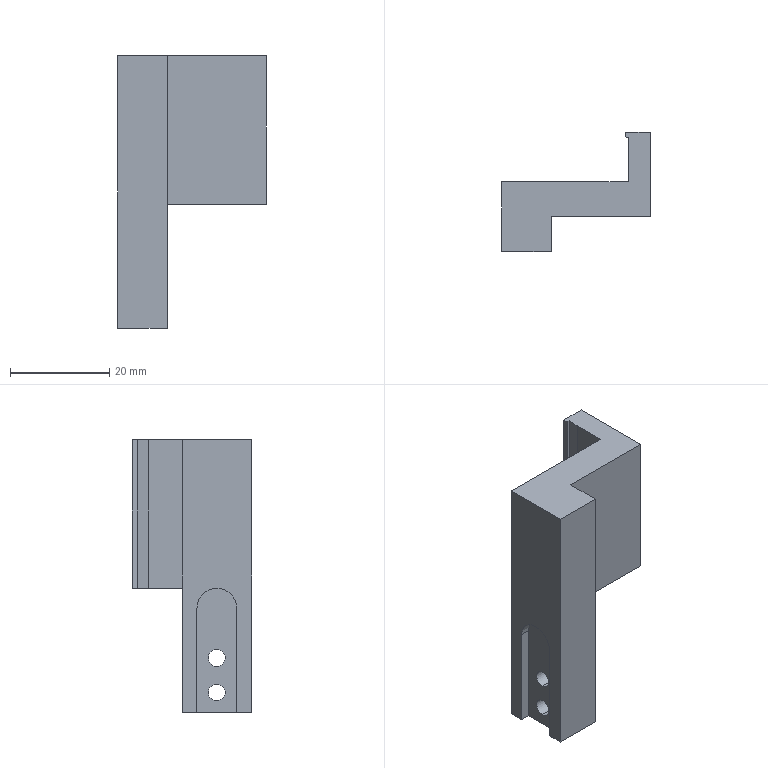Part | STEP file | X77-02303 | 1 solid | 29 faces | box 30 x 24 x 55 mm | volume 12596 mm3 | plane 19 | cylinder 10 | commonest cylinder face diameters 3.4 x4 6 x4 8 x2
STEP:
#1=CARTESIAN_POINT('',(-12.892,-52.894,-18.));
#2=VERTEX_POINT('',#1);
#3=CARTESIAN_POINT('',(-12.892,-52.894,-24.));
#4=VERTEX_POINT('',#3);
#5=CARTESIAN_POINT('',(-12.892,-52.894,-21.));
#6=DIRECTION('',(1.,0.,0.));
#7=DIRECTION('',(0.,0.,-1.));
#8=AXIS2_PLACEMENT_3D('',#5,#6,#7);
#9=CIRCLE('',#8,3.);
#10=EDGE_CURVE('',#2,#4,#9,.T.);
#11=ORIENTED_EDGE('',*,*,#10,.F.);
#12=CARTESIAN_POINT('',(-9.492,-52.894,-18.));
#13=VERTEX_POINT('',#12);
#14=CARTESIAN_POINT('',(-9.492,-52.894,-18.));
#15=DIRECTION('',(1.,0.,0.));
#16=VECTOR('',#15,1000.);
#17=LINE('',#14,#16);
#18=EDGE_CURVE('',#2,#13,#17,.T.);
#19=ORIENTED_EDGE('',*,*,#18,.T.);
#20=CARTESIAN_POINT('',(-9.492,-52.894,-24.));
#21=VERTEX_POINT('',#20);
#22=CARTESIAN_POINT('',(-9.492,-52.894,-21.));
#23=DIRECTION('',(1.,0.,0.));
#24=DIRECTION('',(0.,0.,-1.));
#25=AXIS2_PLACEMENT_3D('',#22,#23,#24);
#26=CIRCLE('',#25,3.);
#27=EDGE_CURVE('',#13,#21,#26,.T.);
#28=ORIENTED_EDGE('',*,*,#27,.T.);
#29=CARTESIAN_POINT('',(-9.492,-52.894,-24.));
#30=DIRECTION('',(1.,0.,0.));
#31=VECTOR('',#30,1000.);
#32=LINE('',#29,#31);
#33=EDGE_CURVE('',#4,#21,#32,.T.);
#34=ORIENTED_EDGE('',*,*,#33,.F.);
#35=EDGE_LOOP('',(#11,#19,#28,#34));
#36=FACE_OUTER_BOUND('',#35,.T.);
#37=CARTESIAN_POINT('',(-9.492,-52.894,-21.));
#38=DIRECTION('',(1.,0.,0.));
#39=DIRECTION('',(0.,0.,-1.));
#40=AXIS2_PLACEMENT_3D('',#37,#38,#39);
#41=CYLINDRICAL_SURFACE('',#40,3.);
#42=ADVANCED_FACE('',(#36),#41,.F.);
#43=CARTESIAN_POINT('',(-17.492,-52.894,-19.3));
#44=VERTEX_POINT('',#43);
#45=CARTESIAN_POINT('',(-17.492,-52.894,-22.7));
#46=VERTEX_POINT('',#45);
#47=CARTESIAN_POINT('',(-17.492,-52.894,-21.));
#48=DIRECTION('',(1.,0.,0.));
#49=DIRECTION('',(0.,0.,-1.));
#50=AXIS2_PLACEMENT_3D('',#47,#48,#49);
#51=CIRCLE('',#50,1.7);
#52=EDGE_CURVE('',#44,#46,#51,.T.);
#53=ORIENTED_EDGE('',*,*,#52,.F.);
#54=CARTESIAN_POINT('',(-12.892,-52.894,-19.3));
#55=VERTEX_POINT('',#54);
#56=CARTESIAN_POINT('',(-9.492,-52.894,-19.3));
#57=DIRECTION('',(1.,0.,0.));
#58=VECTOR('',#57,1000.);
#59=LINE('',#56,#58);
#60=EDGE_CURVE('',#44,#55,#59,.T.);
#61=ORIENTED_EDGE('',*,*,#60,.T.);
#62=CARTESIAN_POINT('',(-12.892,-52.894,-22.7));
#63=VERTEX_POINT('',#62);
#64=CARTESIAN_POINT('',(-12.892,-52.894,-21.));
#65=DIRECTION('',(1.,0.,0.));
#66=DIRECTION('',(0.,0.,-1.));
#67=AXIS2_PLACEMENT_3D('',#64,#65,#66);
#68=CIRCLE('',#67,1.7);
#69=EDGE_CURVE('',#55,#63,#68,.T.);
#70=ORIENTED_EDGE('',*,*,#69,.T.);
#71=CARTESIAN_POINT('',(-9.492,-52.894,-22.7));
#72=DIRECTION('',(1.,0.,0.));
#73=VECTOR('',#72,1000.);
#74=LINE('',#71,#73);
#75=EDGE_CURVE('',#46,#63,#74,.T.);
#76=ORIENTED_EDGE('',*,*,#75,.F.);
#77=EDGE_LOOP('',(#53,#61,#70,#76));
#78=FACE_OUTER_BOUND('',#77,.T.);
#79=CARTESIAN_POINT('',(-9.492,-52.894,-21.));
#80=DIRECTION('',(1.,0.,0.));
#81=DIRECTION('',(0.,0.,-1.));
#82=AXIS2_PLACEMENT_3D('',#79,#80,#81);
#83=CYLINDRICAL_SURFACE('',#82,1.7);
#84=ADVANCED_FACE('',(#78),#83,.F.);
#85=CARTESIAN_POINT('',(-12.892,-52.894,-11.));
#86=VERTEX_POINT('',#85);
#87=CARTESIAN_POINT('',(-12.892,-52.894,-17.));
#88=VERTEX_POINT('',#87);
#89=CARTESIAN_POINT('',(-12.892,-52.894,-14.));
#90=DIRECTION('',(1.,0.,0.));
#91=DIRECTION('',(0.,0.,-1.));
#92=AXIS2_PLACEMENT_3D('',#89,#90,#91);
#93=CIRCLE('',#92,3.);
#94=EDGE_CURVE('',#86,#88,#93,.T.);
#95=ORIENTED_EDGE('',*,*,#94,.F.);
#96=CARTESIAN_POINT('',(-9.492,-52.894,-11.));
#97=VERTEX_POINT('',#96);
#98=CARTESIAN_POINT('',(-9.492,-52.894,-11.));
#99=DIRECTION('',(1.,0.,0.));
#100=VECTOR('',#99,1000.);
#101=LINE('',#98,#100);
#102=EDGE_CURVE('',#86,#97,#101,.T.);
#103=ORIENTED_EDGE('',*,*,#102,.T.);
#104=CARTESIAN_POINT('',(-9.492,-52.894,-17.));
#105=VERTEX_POINT('',#104);
#106=CARTESIAN_POINT('',(-9.492,-52.894,-14.));
#107=DIRECTION('',(1.,0.,0.));
#108=DIRECTION('',(0.,0.,-1.));
#109=AXIS2_PLACEMENT_3D('',#106,#107,#108);
#110=CIRCLE('',#109,3.);
#111=EDGE_CURVE('',#97,#105,#110,.T.);
#112=ORIENTED_EDGE('',*,*,#111,.T.);
#113=CARTESIAN_POINT('',(-9.492,-52.894,-17.));
#114=DIRECTION('',(1.,0.,0.));
#115=VECTOR('',#114,1000.);
#116=LINE('',#113,#115);
#117=EDGE_CURVE('',#88,#105,#116,.T.);
#118=ORIENTED_EDGE('',*,*,#117,.F.);
#119=EDGE_LOOP('',(#95,#103,#112,#118));
#120=FACE_OUTER_BOUND('',#119,.T.);
#121=CARTESIAN_POINT('',(-9.492,-52.894,-14.));
#122=DIRECTION('',(1.,0.,0.));
#123=DIRECTION('',(0.,0.,-1.));
#124=AXIS2_PLACEMENT_3D('',#121,#122,#123);
#125=CYLINDRICAL_SURFACE('',#124,3.);
#126=ADVANCED_FACE('',(#120),#125,.F.);
#127=CARTESIAN_POINT('',(-17.492,-52.894,-12.3));
#128=VERTEX_POINT('',#127);
#129=CARTESIAN_POINT('',(-17.492,-52.894,-15.7));
#130=VERTEX_POINT('',#129);
#131=CARTESIAN_POINT('',(-17.492,-52.894,-14.));
#132=DIRECTION('',(1.,0.,0.));
#133=DIRECTION('',(0.,0.,-1.));
#134=AXIS2_PLACEMENT_3D('',#131,#132,#133);
#135=CIRCLE('',#134,1.7);
#136=EDGE_CURVE('',#128,#130,#135,.T.);
#137=ORIENTED_EDGE('',*,*,#136,.F.);
#138=CARTESIAN_POINT('',(-12.892,-52.894,-12.3));
#139=VERTEX_POINT('',#138);
#140=CARTESIAN_POINT('',(-9.492,-52.894,-12.3));
#141=DIRECTION('',(1.,0.,0.));
#142=VECTOR('',#141,1000.);
#143=LINE('',#140,#142);
#144=EDGE_CURVE('',#128,#139,#143,.T.);
#145=ORIENTED_EDGE('',*,*,#144,.T.);
#146=CARTESIAN_POINT('',(-12.892,-52.894,-15.7));
#147=VERTEX_POINT('',#146);
#148=CARTESIAN_POINT('',(-12.892,-52.894,-14.));
#149=DIRECTION('',(1.,0.,0.));
#150=DIRECTION('',(0.,0.,-1.));
#151=AXIS2_PLACEMENT_3D('',#148,#149,#150);
#152=CIRCLE('',#151,1.7);
#153=EDGE_CURVE('',#139,#147,#152,.T.);
#154=ORIENTED_EDGE('',*,*,#153,.T.);
#155=CARTESIAN_POINT('',(-9.492,-52.894,-15.7));
#156=DIRECTION('',(1.,0.,0.));
#157=VECTOR('',#156,1000.);
#158=LINE('',#155,#157);
#159=EDGE_CURVE('',#130,#147,#158,.T.);
#160=ORIENTED_EDGE('',*,*,#159,.F.);
#161=EDGE_LOOP('',(#137,#145,#154,#160));
#162=FACE_OUTER_BOUND('',#161,.T.);
#163=CARTESIAN_POINT('',(-9.492,-52.894,-14.));
#164=DIRECTION('',(1.,0.,0.));
#165=DIRECTION('',(0.,0.,-1.));
#166=AXIS2_PLACEMENT_3D('',#163,#164,#165);
#167=CYLINDRICAL_SURFACE('',#166,1.7);
#168=ADVANCED_FACE('',(#162),#167,.F.);
#169=CARTESIAN_POINT('',(10.508,-52.894,0.));
#170=VERTEX_POINT('',#169);
#171=CARTESIAN_POINT('',(10.508,-35.894,0.));
#172=VERTEX_POINT('',#171);
#173=CARTESIAN_POINT('',(10.508,-59.894,0.));
#174=DIRECTION('',(0.,1.,0.));
#175=VECTOR('',#174,1000.);
#176=LINE('',#173,#175);
#177=EDGE_CURVE('',#170,#172,#176,.T.);
#178=ORIENTED_EDGE('',*,*,#177,.F.);
#179=CARTESIAN_POINT('',(-9.492,-52.894,0.));
#180=VERTEX_POINT('',#179);
#181=CARTESIAN_POINT('',(-9.492,-52.894,0.));
#182=DIRECTION('',(1.,0.,0.));
#183=VECTOR('',#182,1000.);
#184=LINE('',#181,#183);
#185=EDGE_CURVE('',#180,#170,#184,.T.);
#186=ORIENTED_EDGE('',*,*,#185,.F.);
#187=CARTESIAN_POINT('',(-9.492,-45.894,0.));
#188=VERTEX_POINT('',#187);
#189=CARTESIAN_POINT('',(-9.492,-45.894,0.));
#190=DIRECTION('',(0.,-1.,0.));
#191=VECTOR('',#190,1000.);
#192=LINE('',#189,#191);
#193=EDGE_CURVE('',#188,#180,#192,.T.);
#194=ORIENTED_EDGE('',*,*,#193,.F.);
#195=CARTESIAN_POINT('',(6.008,-45.894,0.));
#196=VERTEX_POINT('',#195);
#197=CARTESIAN_POINT('',(-19.492,-45.894,0.));
#198=DIRECTION('',(1.,0.,0.));
#199=VECTOR('',#198,1000.);
#200=LINE('',#197,#199);
#201=EDGE_CURVE('',#188,#196,#200,.T.);
#202=ORIENTED_EDGE('',*,*,#201,.T.);
#203=CARTESIAN_POINT('',(6.008,-39.22,0.));
#204=VERTEX_POINT('',#203);
#205=CARTESIAN_POINT('',(6.008,-39.22,0.));
#206=DIRECTION('',(0.,-1.,0.));
#207=VECTOR('',#206,1000.);
#208=LINE('',#205,#207);
#209=EDGE_CURVE('',#204,#196,#208,.T.);
#210=ORIENTED_EDGE('',*,*,#209,.F.);
#211=CARTESIAN_POINT('',(6.165,-36.894,0.));
#212=VERTEX_POINT('',#211);
#213=CARTESIAN_POINT('',(6.165,-36.894,0.));
#214=DIRECTION('',(-0.06762,-0.9977,0.));
#215=VECTOR('',#214,1000.);
#216=LINE('',#213,#215);
#217=EDGE_CURVE('',#212,#204,#216,.T.);
#218=ORIENTED_EDGE('',*,*,#217,.F.);
#219=CARTESIAN_POINT('',(5.595,-36.894,0.));
#220=VERTEX_POINT('',#219);
#221=CARTESIAN_POINT('',(5.595,-36.894,0.));
#222=DIRECTION('',(1.,0.,0.));
#223=VECTOR('',#222,1000.);
#224=LINE('',#221,#223);
#225=EDGE_CURVE('',#220,#212,#224,.T.);
#226=ORIENTED_EDGE('',*,*,#225,.F.);
#227=CARTESIAN_POINT('',(5.508,-35.894,0.));
#228=VERTEX_POINT('',#227);
#229=CARTESIAN_POINT('',(5.508,-35.894,0.));
#230=DIRECTION('',(0.08716,-0.9962,0.));
#231=VECTOR('',#230,1000.);
#232=LINE('',#229,#231);
#233=EDGE_CURVE('',#228,#220,#232,.T.);
#234=ORIENTED_EDGE('',*,*,#233,.F.);
#235=CARTESIAN_POINT('',(10.508,-35.894,0.));
#236=DIRECTION('',(-1.,0.,0.));
#237=VECTOR('',#236,1000.);
#238=LINE('',#235,#237);
#239=EDGE_CURVE('',#172,#228,#238,.T.);
#240=ORIENTED_EDGE('',*,*,#239,.F.);
#241=EDGE_LOOP('',(#178,#186,#194,#202,#210,#218,#226,#234,#240));
#242=FACE_OUTER_BOUND('',#241,.T.);
#243=CARTESIAN_POINT('',(10.508,-35.894,0.));
#244=DIRECTION('',(0.,0.,1.));
#245=DIRECTION('',(1.,0.,0.));
#246=AXIS2_PLACEMENT_3D('',#243,#244,#245);
#247=PLANE('',#246);
#248=ADVANCED_FACE('',(#242),#247,.F.);
#249=CARTESIAN_POINT('',(6.008,-45.894,30.));
#250=VERTEX_POINT('',#249);
#251=CARTESIAN_POINT('',(6.008,-45.894,0.));
#252=DIRECTION('',(0.,0.,-1.));
#253=VECTOR('',#252,1000.);
#254=LINE('',#251,#253);
#255=EDGE_CURVE('',#250,#196,#254,.T.);
#256=ORIENTED_EDGE('',*,*,#255,.F.);
#257=CARTESIAN_POINT('',(6.008,-39.22,30.));
#258=VERTEX_POINT('',#257);
#259=CARTESIAN_POINT('',(6.008,-39.22,30.));
#260=DIRECTION('',(0.,-1.,0.));
#261=VECTOR('',#260,1000.);
#262=LINE('',#259,#261);
#263=EDGE_CURVE('',#258,#250,#262,.T.);
#264=ORIENTED_EDGE('',*,*,#263,.F.);
#265=CARTESIAN_POINT('',(6.008,-39.22,30.));
#266=DIRECTION('',(0.,0.,-1.));
#267=VECTOR('',#266,1000.);
#268=LINE('',#265,#267);
#269=EDGE_CURVE('',#258,#204,#268,.T.);
#270=ORIENTED_EDGE('',*,*,#269,.T.);
#271=ORIENTED_EDGE('',*,*,#209,.T.);
#272=EDGE_LOOP('',(#256,#264,#270,#271));
#273=FACE_OUTER_BOUND('',#272,.T.);
#274=CARTESIAN_POINT('',(6.008,-39.22,30.));
#275=DIRECTION('',(1.,0.,0.));
#276=DIRECTION('',(0.,0.,-1.));
#277=AXIS2_PLACEMENT_3D('',#274,#275,#276);
#278=PLANE('',#277);
#279=ADVANCED_FACE('',(#273),#278,.F.);
#280=CARTESIAN_POINT('',(10.508,-52.894,30.));
#281=VERTEX_POINT('',#280);
#282=CARTESIAN_POINT('',(10.508,-35.894,30.));
#283=VERTEX_POINT('',#282);
#284=CARTESIAN_POINT('',(10.508,-59.894,30.));
#285=DIRECTION('',(0.,1.,0.));
#286=VECTOR('',#285,1000.);
#287=LINE('',#284,#286);
#288=EDGE_CURVE('',#281,#283,#287,.T.);
#289=ORIENTED_EDGE('',*,*,#288,.F.);
#290=CARTESIAN_POINT('',(10.508,-52.894,30.));
#291=DIRECTION('',(0.,0.,-1.));
#292=VECTOR('',#291,1000.);
#293=LINE('',#290,#292);
#294=EDGE_CURVE('',#281,#170,#293,.T.);
#295=ORIENTED_EDGE('',*,*,#294,.T.);
#296=ORIENTED_EDGE('',*,*,#177,.T.);
#297=CARTESIAN_POINT('',(10.508,-35.894,30.));
#298=DIRECTION('',(0.,0.,-1.));
#299=VECTOR('',#298,1000.);
#300=LINE('',#297,#299);
#301=EDGE_CURVE('',#283,#172,#300,.T.);
#302=ORIENTED_EDGE('',*,*,#301,.F.);
#303=EDGE_LOOP('',(#289,#295,#296,#302));
#304=FACE_OUTER_BOUND('',#303,.T.);
#305=CARTESIAN_POINT('',(10.508,-59.894,30.));
#306=DIRECTION('',(-1.,0.,0.));
#307=DIRECTION('',(0.,-1.,0.));
#308=AXIS2_PLACEMENT_3D('',#305,#306,#307);
#309=PLANE('',#308);
#310=ADVANCED_FACE('',(#304),#309,.F.);
#311=ORIENTED_EDGE('',*,*,#239,.T.);
#312=CARTESIAN_POINT('',(5.508,-35.894,30.));
#313=VERTEX_POINT('',#312);
#314=CARTESIAN_POINT('',(5.508,-35.894,30.));
#315=DIRECTION('',(0.,0.,-1.));
#316=VECTOR('',#315,1000.);
#317=LINE('',#314,#316);
#318=EDGE_CURVE('',#313,#228,#317,.T.);
#319=ORIENTED_EDGE('',*,*,#318,.F.);
#320=CARTESIAN_POINT('',(10.508,-35.894,30.));
#321=DIRECTION('',(-1.,0.,0.));
#322=VECTOR('',#321,1000.);
#323=LINE('',#320,#322);
#324=EDGE_CURVE('',#283,#313,#323,.T.);
#325=ORIENTED_EDGE('',*,*,#324,.F.);
#326=ORIENTED_EDGE('',*,*,#301,.T.);
#327=EDGE_LOOP('',(#311,#319,#325,#326));
#328=FACE_OUTER_BOUND('',#327,.T.);
#329=CARTESIAN_POINT('',(10.508,-35.894,30.));
#330=DIRECTION('',(0.,-1.,0.));
#331=DIRECTION('',(0.,0.,-1.));
#332=AXIS2_PLACEMENT_3D('',#329,#330,#331);
#333=PLANE('',#332);
#334=ADVANCED_FACE('',(#328),#333,.F.);
#335=ORIENTED_EDGE('',*,*,#233,.T.);
#336=CARTESIAN_POINT('',(5.595,-36.894,30.));
#337=VERTEX_POINT('',#336);
#338=CARTESIAN_POINT('',(5.595,-36.894,30.));
#339=DIRECTION('',(0.,0.,-1.));
#340=VECTOR('',#339,1000.);
#341=LINE('',#338,#340);
#342=EDGE_CURVE('',#337,#220,#341,.T.);
#343=ORIENTED_EDGE('',*,*,#342,.F.);
#344=CARTESIAN_POINT('',(5.508,-35.894,30.));
#345=DIRECTION('',(0.08716,-0.9962,0.));
#346=VECTOR('',#345,1000.);
#347=LINE('',#344,#346);
#348=EDGE_CURVE('',#313,#337,#347,.T.);
#349=ORIENTED_EDGE('',*,*,#348,.F.);
#350=ORIENTED_EDGE('',*,*,#318,.T.);
#351=EDGE_LOOP('',(#335,#343,#349,#350));
#352=FACE_OUTER_BOUND('',#351,.T.);
#353=CARTESIAN_POINT('',(5.508,-35.894,30.));
#354=DIRECTION('',(0.9962,0.08716,0.));
#355=DIRECTION('',(-0.08716,0.9962,0.));
#356=AXIS2_PLACEMENT_3D('',#353,#354,#355);
#357=PLANE('',#356);
#358=ADVANCED_FACE('',(#352),#357,.F.);
#359=ORIENTED_EDGE('',*,*,#225,.T.);
#360=CARTESIAN_POINT('',(6.165,-36.894,30.));
#361=VERTEX_POINT('',#360);
#362=CARTESIAN_POINT('',(6.165,-36.894,30.));
#363=DIRECTION('',(0.,0.,-1.));
#364=VECTOR('',#363,1000.);
#365=LINE('',#362,#364);
#366=EDGE_CURVE('',#361,#212,#365,.T.);
#367=ORIENTED_EDGE('',*,*,#366,.F.);
#368=CARTESIAN_POINT('',(5.595,-36.894,30.));
#369=DIRECTION('',(1.,0.,0.));
#370=VECTOR('',#369,1000.);
#371=LINE('',#368,#370);
#372=EDGE_CURVE('',#337,#361,#371,.T.);
#373=ORIENTED_EDGE('',*,*,#372,.F.);
#374=ORIENTED_EDGE('',*,*,#342,.T.);
#375=EDGE_LOOP('',(#359,#367,#373,#374));
#376=FACE_OUTER_BOUND('',#375,.T.);
#377=CARTESIAN_POINT('',(5.595,-36.894,30.));
#378=DIRECTION('',(0.,1.,0.));
#379=DIRECTION('',(0.,0.,1.));
#380=AXIS2_PLACEMENT_3D('',#377,#378,#379);
#381=PLANE('',#380);
#382=ADVANCED_FACE('',(#376),#381,.F.);
#383=ORIENTED_EDGE('',*,*,#217,.T.);
#384=ORIENTED_EDGE('',*,*,#269,.F.);
#385=CARTESIAN_POINT('',(6.165,-36.894,30.));
#386=DIRECTION('',(-0.06762,-0.9977,0.));
#387=VECTOR('',#386,1000.);
#388=LINE('',#385,#387);
#389=EDGE_CURVE('',#361,#258,#388,.T.);
#390=ORIENTED_EDGE('',*,*,#389,.F.);
#391=ORIENTED_EDGE('',*,*,#366,.T.);
#392=EDGE_LOOP('',(#383,#384,#390,#391));
#393=FACE_OUTER_BOUND('',#392,.T.);
#394=CARTESIAN_POINT('',(6.165,-36.894,30.));
#395=DIRECTION('',(0.9977,-0.06762,0.));
#396=DIRECTION('',(0.06762,0.9977,0.));
#397=AXIS2_PLACEMENT_3D('',#394,#395,#396);
#398=PLANE('',#397);
#399=ADVANCED_FACE('',(#393),#398,.F.);
#400=CARTESIAN_POINT('',(-9.492,-59.894,-25.));
#401=VERTEX_POINT('',#400);
#402=CARTESIAN_POINT('',(-9.492,-59.894,30.));
#403=VERTEX_POINT('',#402);
#404=CARTESIAN_POINT('',(-9.492,-59.894,-25.));
#405=DIRECTION('',(0.,0.,1.));
#406=VECTOR('',#405,1000.);
#407=LINE('',#404,#406);
#408=EDGE_CURVE('',#401,#403,#407,.T.);
#409=ORIENTED_EDGE('',*,*,#408,.T.);
#410=CARTESIAN_POINT('',(-19.492,-59.894,30.));
#411=VERTEX_POINT('',#410);
#412=CARTESIAN_POINT('',(6.008,-59.894,30.));
#413=DIRECTION('',(1.,0.,0.));
#414=VECTOR('',#413,1000.);
#415=LINE('',#412,#414);
#416=EDGE_CURVE('',#411,#403,#415,.T.);
#417=ORIENTED_EDGE('',*,*,#416,.F.);
#418=CARTESIAN_POINT('',(-19.492,-59.894,-25.));
#419=VERTEX_POINT('',#418);
#420=CARTESIAN_POINT('',(-19.492,-59.894,0.));
#421=DIRECTION('',(0.,0.,1.));
#422=VECTOR('',#421,1000.);
#423=LINE('',#420,#422);
#424=EDGE_CURVE('',#419,#411,#423,.T.);
#425=ORIENTED_EDGE('',*,*,#424,.F.);
#426=CARTESIAN_POINT('',(-19.492,-59.894,-25.));
#427=DIRECTION('',(-1.,0.,0.));
#428=VECTOR('',#427,1000.);
#429=LINE('',#426,#428);
#430=EDGE_CURVE('',#401,#419,#429,.T.);
#431=ORIENTED_EDGE('',*,*,#430,.F.);
#432=EDGE_LOOP('',(#409,#417,#425,#431));
#433=FACE_OUTER_BOUND('',#432,.T.);
#434=CARTESIAN_POINT('',(6.008,-59.894,30.));
#435=DIRECTION('',(0.,1.,0.));
#436=DIRECTION('',(0.,0.,1.));
#437=AXIS2_PLACEMENT_3D('',#434,#435,#436);
#438=PLANE('',#437);
#439=ADVANCED_FACE('',(#433),#438,.F.);
#440=CARTESIAN_POINT('',(-9.492,-52.894,30.));
#441=VERTEX_POINT('',#440);
#442=CARTESIAN_POINT('',(-9.492,-59.894,30.));
#443=DIRECTION('',(0.,1.,0.));
#444=VECTOR('',#443,1000.);
#445=LINE('',#442,#444);
#446=EDGE_CURVE('',#403,#441,#445,.T.);
#447=ORIENTED_EDGE('',*,*,#446,.T.);
#448=CARTESIAN_POINT('',(-9.492,-52.894,30.));
#449=DIRECTION('',(1.,0.,0.));
#450=VECTOR('',#449,1000.);
#451=LINE('',#448,#450);
#452=EDGE_CURVE('',#441,#281,#451,.T.);
#453=ORIENTED_EDGE('',*,*,#452,.T.);
#454=ORIENTED_EDGE('',*,*,#288,.T.);
#455=ORIENTED_EDGE('',*,*,#324,.T.);
#456=ORIENTED_EDGE('',*,*,#348,.T.);
#457=ORIENTED_EDGE('',*,*,#372,.T.);
#458=ORIENTED_EDGE('',*,*,#389,.T.);
#459=ORIENTED_EDGE('',*,*,#263,.T.);
#460=CARTESIAN_POINT('',(-19.492,-45.894,30.));
#461=VERTEX_POINT('',#460);
#462=CARTESIAN_POINT('',(-19.492,-45.894,30.));
#463=DIRECTION('',(1.,0.,0.));
#464=VECTOR('',#463,1000.);
#465=LINE('',#462,#464);
#466=EDGE_CURVE('',#461,#250,#465,.T.);
#467=ORIENTED_EDGE('',*,*,#466,.F.);
#468=CARTESIAN_POINT('',(-19.492,-45.894,30.));
#469=DIRECTION('',(0.,1.,0.));
#470=VECTOR('',#469,1000.);
#471=LINE('',#468,#470);
#472=EDGE_CURVE('',#411,#461,#471,.T.);
#473=ORIENTED_EDGE('',*,*,#472,.F.);
#474=ORIENTED_EDGE('',*,*,#416,.T.);
#475=EDGE_LOOP('',(#447,#453,#454,#455,#456,#457,#458,#459,#467,#473,#474));
#476=FACE_OUTER_BOUND('',#475,.T.);
#477=CARTESIAN_POINT('',(10.508,-35.894,30.));
#478=DIRECTION('',(0.,0.,1.));
#479=DIRECTION('',(1.,0.,0.));
#480=AXIS2_PLACEMENT_3D('',#477,#478,#479);
#481=PLANE('',#480);
#482=ADVANCED_FACE('',(#476),#481,.T.);
#483=ORIENTED_EDGE('',*,*,#255,.T.);
#484=ORIENTED_EDGE('',*,*,#201,.F.);
#485=CARTESIAN_POINT('',(-9.492,-45.894,-25.));
#486=VERTEX_POINT('',#485);
#487=CARTESIAN_POINT('',(-9.492,-45.894,-25.));
#488=DIRECTION('',(0.,0.,1.));
#489=VECTOR('',#488,1000.);
#490=LINE('',#487,#489);
#491=EDGE_CURVE('',#486,#188,#490,.T.);
#492=ORIENTED_EDGE('',*,*,#491,.F.);
#493=CARTESIAN_POINT('',(-19.492,-45.894,-25.));
#494=VERTEX_POINT('',#493);
#495=CARTESIAN_POINT('',(-19.492,-45.894,-25.));
#496=DIRECTION('',(1.,0.,0.));
#497=VECTOR('',#496,1000.);
#498=LINE('',#495,#497);
#499=EDGE_CURVE('',#494,#486,#498,.T.);
#500=ORIENTED_EDGE('',*,*,#499,.F.);
#501=CARTESIAN_POINT('',(-19.492,-45.894,0.));
#502=DIRECTION('',(0.,0.,-1.));
#503=VECTOR('',#502,1000.);
#504=LINE('',#501,#503);
#505=EDGE_CURVE('',#461,#494,#504,.T.);
#506=ORIENTED_EDGE('',*,*,#505,.F.);
#507=ORIENTED_EDGE('',*,*,#466,.T.);
#508=EDGE_LOOP('',(#483,#484,#492,#500,#506,#507));
#509=FACE_OUTER_BOUND('',#508,.T.);
#510=CARTESIAN_POINT('',(-19.492,-45.894,0.));
#511=DIRECTION('',(0.,-1.,0.));
#512=DIRECTION('',(0.,0.,-1.));
#513=AXIS2_PLACEMENT_3D('',#510,#511,#512);
#514=PLANE('',#513);
#515=ADVANCED_FACE('',(#509),#514,.F.);
#516=CARTESIAN_POINT('',(-19.492,-48.894,-4.));
#517=VERTEX_POINT('',#516);
#518=CARTESIAN_POINT('',(-19.492,-48.894,-25.));
#519=VERTEX_POINT('',#518);
#520=CARTESIAN_POINT('',(-19.492,-48.894,0.));
#521=DIRECTION('',(0.,0.,-1.));
#522=VECTOR('',#521,1000.);
#523=LINE('',#520,#522);
#524=EDGE_CURVE('',#517,#519,#523,.T.);
#525=ORIENTED_EDGE('',*,*,#524,.F.);
#526=CARTESIAN_POINT('',(-19.492,-52.894,0.));
#527=VERTEX_POINT('',#526);
#528=CARTESIAN_POINT('',(-19.492,-52.894,-4.));
#529=DIRECTION('',(1.,0.,0.));
#530=DIRECTION('',(0.,0.,1.));
#531=AXIS2_PLACEMENT_3D('',#528,#529,#530);
#532=CIRCLE('',#531,4.);
#533=EDGE_CURVE('',#517,#527,#532,.T.);
#534=ORIENTED_EDGE('',*,*,#533,.T.);
#535=CARTESIAN_POINT('',(-19.492,-56.894,-4.));
#536=VERTEX_POINT('',#535);
#537=CARTESIAN_POINT('',(-19.492,-52.894,-4.));
#538=DIRECTION('',(1.,0.,0.));
#539=DIRECTION('',(0.,0.,1.));
#540=AXIS2_PLACEMENT_3D('',#537,#538,#539);
#541=CIRCLE('',#540,4.);
#542=EDGE_CURVE('',#527,#536,#541,.T.);
#543=ORIENTED_EDGE('',*,*,#542,.T.);
#544=CARTESIAN_POINT('',(-19.492,-56.894,-25.));
#545=VERTEX_POINT('',#544);
#546=CARTESIAN_POINT('',(-19.492,-56.894,0.));
#547=DIRECTION('',(0.,0.,1.));
#548=VECTOR('',#547,1000.);
#549=LINE('',#546,#548);
#550=EDGE_CURVE('',#545,#536,#549,.T.);
#551=ORIENTED_EDGE('',*,*,#550,.F.);
#552=CARTESIAN_POINT('',(-19.492,-45.894,-25.));
#553=DIRECTION('',(0.,1.,0.));
#554=VECTOR('',#553,1000.);
#555=LINE('',#552,#554);
#556=EDGE_CURVE('',#419,#545,#555,.T.);
#557=ORIENTED_EDGE('',*,*,#556,.F.);
#558=ORIENTED_EDGE('',*,*,#424,.T.);
#559=ORIENTED_EDGE('',*,*,#472,.T.);
#560=ORIENTED_EDGE('',*,*,#505,.T.);
#561=CARTESIAN_POINT('',(-19.492,-45.894,-25.));
#562=DIRECTION('',(0.,1.,0.));
#563=VECTOR('',#562,1000.);
#564=LINE('',#561,#563);
#565=EDGE_CURVE('',#519,#494,#564,.T.);
#566=ORIENTED_EDGE('',*,*,#565,.F.);
#567=EDGE_LOOP('',(#525,#534,#543,#551,#557,#558,#559,#560,#566));
#568=FACE_OUTER_BOUND('',#567,.T.);
#569=CARTESIAN_POINT('',(-19.492,-59.894,0.));
#570=DIRECTION('',(-1.,0.,0.));
#571=DIRECTION('',(0.,0.,1.));
#572=AXIS2_PLACEMENT_3D('',#569,#570,#571);
#573=PLANE('',#572);
#574=ADVANCED_FACE('',(#568),#573,.T.);
#575=CARTESIAN_POINT('',(-9.492,-52.894,-21.));
#576=DIRECTION('',(1.,0.,0.));
#577=DIRECTION('',(0.,0.,-1.));
#578=AXIS2_PLACEMENT_3D('',#575,#576,#577);
#579=CIRCLE('',#578,3.);
#580=EDGE_CURVE('',#21,#13,#579,.T.);
#581=ORIENTED_EDGE('',*,*,#580,.F.);
#582=ORIENTED_EDGE('',*,*,#27,.F.);
#583=EDGE_LOOP('',(#581,#582));
#584=FACE_BOUND('',#583,.T.);
#585=CARTESIAN_POINT('',(-9.492,-52.894,-14.));
#586=DIRECTION('',(1.,0.,0.));
#587=DIRECTION('',(0.,0.,-1.));
#588=AXIS2_PLACEMENT_3D('',#585,#586,#587);
#589=CIRCLE('',#588,3.);
#590=EDGE_CURVE('',#105,#97,#589,.T.);
#591=ORIENTED_EDGE('',*,*,#590,.F.);
#592=ORIENTED_EDGE('',*,*,#111,.F.);
#593=EDGE_LOOP('',(#591,#592));
#594=FACE_BOUND('',#593,.T.);
#595=ORIENTED_EDGE('',*,*,#193,.T.);
#596=CARTESIAN_POINT('',(-9.492,-52.894,30.));
#597=DIRECTION('',(0.,0.,-1.));
#598=VECTOR('',#597,1000.);
#599=LINE('',#596,#598);
#600=EDGE_CURVE('',#441,#180,#599,.T.);
#601=ORIENTED_EDGE('',*,*,#600,.F.);
#602=ORIENTED_EDGE('',*,*,#446,.F.);
#603=ORIENTED_EDGE('',*,*,#408,.F.);
#604=CARTESIAN_POINT('',(-9.492,-45.894,-25.));
#605=DIRECTION('',(0.,-1.,0.));
#606=VECTOR('',#605,1000.);
#607=LINE('',#604,#606);
#608=EDGE_CURVE('',#486,#401,#607,.T.);
#609=ORIENTED_EDGE('',*,*,#608,.F.);
#610=ORIENTED_EDGE('',*,*,#491,.T.);
#611=EDGE_LOOP('',(#595,#601,#602,#603,#609,#610));
#612=FACE_OUTER_BOUND('',#611,.T.);
#613=CARTESIAN_POINT('',(-9.492,-45.894,-25.));
#614=DIRECTION('',(-1.,0.,0.));
#615=DIRECTION('',(0.,-1.,0.));
#616=AXIS2_PLACEMENT_3D('',#613,#614,#615);
#617=PLANE('',#616);
#618=ADVANCED_FACE('',(#584,#594,#612),#617,.F.);
#619=CARTESIAN_POINT('',(-17.492,-56.894,-25.));
#620=VERTEX_POINT('',#619);
#621=CARTESIAN_POINT('',(-17.492,-48.894,-25.));
#622=VERTEX_POINT('',#621);
#623=CARTESIAN_POINT('',(-17.492,-59.894,-25.));
#624=DIRECTION('',(0.,1.,0.));
#625=VECTOR('',#624,1000.);
#626=LINE('',#623,#625);
#627=EDGE_CURVE('',#620,#622,#626,.T.);
#628=ORIENTED_EDGE('',*,*,#627,.T.);
#629=CARTESIAN_POINT('',(-19.492,-48.894,-25.));
#630=DIRECTION('',(-1.,0.,0.));
#631=VECTOR('',#630,1000.);
#632=LINE('',#629,#631);
#633=EDGE_CURVE('',#622,#519,#632,.T.);
#634=ORIENTED_EDGE('',*,*,#633,.T.);
#635=ORIENTED_EDGE('',*,*,#565,.T.);
#636=ORIENTED_EDGE('',*,*,#499,.T.);
#637=ORIENTED_EDGE('',*,*,#608,.T.);
#638=ORIENTED_EDGE('',*,*,#430,.T.);
#639=ORIENTED_EDGE('',*,*,#556,.T.);
#640=CARTESIAN_POINT('',(-19.492,-56.894,-25.));
#641=DIRECTION('',(1.,0.,0.));
#642=VECTOR('',#641,1000.);
#643=LINE('',#640,#642);
#644=EDGE_CURVE('',#545,#620,#643,.T.);
#645=ORIENTED_EDGE('',*,*,#644,.T.);
#646=EDGE_LOOP('',(#628,#634,#635,#636,#637,#638,#639,#645));
#647=FACE_OUTER_BOUND('',#646,.T.);
#648=CARTESIAN_POINT('',(-19.492,-59.894,-25.));
#649=DIRECTION('',(0.,0.,1.));
#650=DIRECTION('',(1.,0.,0.));
#651=AXIS2_PLACEMENT_3D('',#648,#649,#650);
#652=PLANE('',#651);
#653=ADVANCED_FACE('',(#647),#652,.F.);
#654=CARTESIAN_POINT('',(-17.492,-52.894,-21.));
#655=DIRECTION('',(1.,0.,0.));
#656=DIRECTION('',(0.,0.,-1.));
#657=AXIS2_PLACEMENT_3D('',#654,#655,#656);
#658=CIRCLE('',#657,1.7);
#659=EDGE_CURVE('',#46,#44,#658,.T.);
#660=ORIENTED_EDGE('',*,*,#659,.T.);
#661=ORIENTED_EDGE('',*,*,#52,.T.);
#662=EDGE_LOOP('',(#660,#661));
#663=FACE_BOUND('',#662,.T.);
#664=CARTESIAN_POINT('',(-17.492,-52.894,-14.));
#665=DIRECTION('',(1.,0.,0.));
#666=DIRECTION('',(0.,0.,-1.));
#667=AXIS2_PLACEMENT_3D('',#664,#665,#666);
#668=CIRCLE('',#667,1.7);
#669=EDGE_CURVE('',#130,#128,#668,.T.);
#670=ORIENTED_EDGE('',*,*,#669,.T.);
#671=ORIENTED_EDGE('',*,*,#136,.T.);
#672=EDGE_LOOP('',(#670,#671));
#673=FACE_BOUND('',#672,.T.);
#674=CARTESIAN_POINT('',(-17.492,-56.894,-4.));
#675=VERTEX_POINT('',#674);
#676=CARTESIAN_POINT('',(-17.492,-56.894,-25.));
#677=DIRECTION('',(0.,0.,1.));
#678=VECTOR('',#677,1000.);
#679=LINE('',#676,#678);
#680=EDGE_CURVE('',#620,#675,#679,.T.);
#681=ORIENTED_EDGE('',*,*,#680,.T.);
#682=CARTESIAN_POINT('',(-17.492,-52.894,0.));
#683=VERTEX_POINT('',#682);
#684=CARTESIAN_POINT('',(-17.492,-52.894,-4.));
#685=DIRECTION('',(-1.,0.,0.));
#686=DIRECTION('',(0.,0.,-1.));
#687=AXIS2_PLACEMENT_3D('',#684,#685,#686);
#688=CIRCLE('',#687,4.);
#689=EDGE_CURVE('',#675,#683,#688,.T.);
#690=ORIENTED_EDGE('',*,*,#689,.T.);
#691=CARTESIAN_POINT('',(-17.492,-48.894,-4.));
#692=VERTEX_POINT('',#691);
#693=CARTESIAN_POINT('',(-17.492,-52.894,-4.));
#694=DIRECTION('',(-1.,0.,0.));
#695=DIRECTION('',(0.,0.,-1.));
#696=AXIS2_PLACEMENT_3D('',#693,#694,#695);
#697=CIRCLE('',#696,4.);
#698=EDGE_CURVE('',#683,#692,#697,.T.);
#699=ORIENTED_EDGE('',*,*,#698,.T.);
#700=CARTESIAN_POINT('',(-17.492,-48.894,-25.));
#701=DIRECTION('',(0.,0.,1.));
#702=VECTOR('',#701,1000.);
#703=LINE('',#700,#702);
#704=EDGE_CURVE('',#622,#692,#703,.T.);
#705=ORIENTED_EDGE('',*,*,#704,.F.);
#706=ORIENTED_EDGE('',*,*,#627,.F.);
#707=EDGE_LOOP('',(#681,#690,#699,#705,#706));
#708=FACE_OUTER_BOUND('',#707,.T.);
#709=CARTESIAN_POINT('',(-17.492,-56.894,-25.));
#710=DIRECTION('',(1.,0.,0.));
#711=DIRECTION('',(0.,0.,-1.));
#712=AXIS2_PLACEMENT_3D('',#709,#710,#711);
#713=PLANE('',#712);
#714=ADVANCED_FACE('',(#663,#673,#708),#713,.F.);
#715=ORIENTED_EDGE('',*,*,#704,.T.);
#716=CARTESIAN_POINT('',(-20.922,-48.894,-4.));
#717=DIRECTION('',(-1.,0.,0.));
#718=VECTOR('',#717,1000.);
#719=LINE('',#716,#718);
#720=EDGE_CURVE('',#692,#517,#719,.T.);
#721=ORIENTED_EDGE('',*,*,#720,.T.);
#722=ORIENTED_EDGE('',*,*,#524,.T.);
#723=ORIENTED_EDGE('',*,*,#633,.F.);
#724=EDGE_LOOP('',(#715,#721,#722,#723));
#725=FACE_OUTER_BOUND('',#724,.T.);
#726=CARTESIAN_POINT('',(-20.922,-48.894,-25.));
#727=DIRECTION('',(0.,1.,0.));
#728=DIRECTION('',(0.,0.,1.));
#729=AXIS2_PLACEMENT_3D('',#726,#727,#728);
#730=PLANE('',#729);
#731=ADVANCED_FACE('',(#725),#730,.F.);
#732=ORIENTED_EDGE('',*,*,#550,.T.);
#733=CARTESIAN_POINT('',(-20.922,-56.894,-4.));
#734=DIRECTION('',(1.,0.,0.));
#735=VECTOR('',#734,1000.);
#736=LINE('',#733,#735);
#737=EDGE_CURVE('',#536,#675,#736,.T.);
#738=ORIENTED_EDGE('',*,*,#737,.T.);
#739=ORIENTED_EDGE('',*,*,#680,.F.);
#740=ORIENTED_EDGE('',*,*,#644,.F.);
#741=EDGE_LOOP('',(#732,#738,#739,#740));
#742=FACE_OUTER_BOUND('',#741,.T.);
#743=CARTESIAN_POINT('',(-20.922,-56.894,-25.));
#744=DIRECTION('',(0.,-1.,0.));
#745=DIRECTION('',(0.,0.,-1.));
#746=AXIS2_PLACEMENT_3D('',#743,#744,#745);
#747=PLANE('',#746);
#748=ADVANCED_FACE('',(#742),#747,.F.);
#749=CARTESIAN_POINT('',(-20.922,-52.894,0.));
#750=DIRECTION('',(1.,0.,0.));
#751=VECTOR('',#750,1000.);
#752=LINE('',#749,#751);
#753=EDGE_CURVE('',#527,#683,#752,.T.);
#754=ORIENTED_EDGE('',*,*,#753,.F.);
#755=ORIENTED_EDGE('',*,*,#533,.F.);
#756=ORIENTED_EDGE('',*,*,#720,.F.);
#757=ORIENTED_EDGE('',*,*,#698,.F.);
#758=EDGE_LOOP('',(#754,#755,#756,#757));
#759=FACE_OUTER_BOUND('',#758,.T.);
#760=CARTESIAN_POINT('',(-20.922,-52.894,-4.));
#761=DIRECTION('',(-1.,0.,0.));
#762=DIRECTION('',(0.,0.,1.));
#763=AXIS2_PLACEMENT_3D('',#760,#761,#762);
#764=CYLINDRICAL_SURFACE('',#763,4.);
#765=ADVANCED_FACE('',(#759),#764,.F.);
#766=ORIENTED_EDGE('',*,*,#542,.F.);
#767=ORIENTED_EDGE('',*,*,#753,.T.);
#768=ORIENTED_EDGE('',*,*,#689,.F.);
#769=ORIENTED_EDGE('',*,*,#737,.F.);
#770=EDGE_LOOP('',(#766,#767,#768,#769));
#771=FACE_OUTER_BOUND('',#770,.T.);
#772=CARTESIAN_POINT('',(-20.922,-52.894,-4.));
#773=DIRECTION('',(1.,0.,0.));
#774=DIRECTION('',(0.,0.,-1.));
#775=AXIS2_PLACEMENT_3D('',#772,#773,#774);
#776=CYLINDRICAL_SURFACE('',#775,4.);
#777=ADVANCED_FACE('',(#771),#776,.F.);
#778=ORIENTED_EDGE('',*,*,#185,.T.);
#779=ORIENTED_EDGE('',*,*,#294,.F.);
#780=ORIENTED_EDGE('',*,*,#452,.F.);
#781=ORIENTED_EDGE('',*,*,#600,.T.);
#782=EDGE_LOOP('',(#778,#779,#780,#781));
#783=FACE_OUTER_BOUND('',#782,.T.);
#784=CARTESIAN_POINT('',(-9.492,-52.894,30.));
#785=DIRECTION('',(0.,1.,0.));
#786=DIRECTION('',(0.,0.,1.));
#787=AXIS2_PLACEMENT_3D('',#784,#785,#786);
#788=PLANE('',#787);
#789=ADVANCED_FACE('',(#783),#788,.F.);
#790=ORIENTED_EDGE('',*,*,#144,.F.);
#791=ORIENTED_EDGE('',*,*,#669,.F.);
#792=ORIENTED_EDGE('',*,*,#159,.T.);
#793=CARTESIAN_POINT('',(-12.892,-52.894,-14.));
#794=DIRECTION('',(1.,0.,0.));
#795=DIRECTION('',(0.,0.,-1.));
#796=AXIS2_PLACEMENT_3D('',#793,#794,#795);
#797=CIRCLE('',#796,1.7);
#798=EDGE_CURVE('',#147,#139,#797,.T.);
#799=ORIENTED_EDGE('',*,*,#798,.T.);
#800=EDGE_LOOP('',(#790,#791,#792,#799));
#801=FACE_OUTER_BOUND('',#800,.T.);
#802=CARTESIAN_POINT('',(-9.492,-52.894,-14.));
#803=DIRECTION('',(1.,0.,0.));
#804=DIRECTION('',(0.,0.,-1.));
#805=AXIS2_PLACEMENT_3D('',#802,#803,#804);
#806=CYLINDRICAL_SURFACE('',#805,1.7);
#807=ADVANCED_FACE('',(#801),#806,.F.);
#808=ORIENTED_EDGE('',*,*,#798,.F.);
#809=ORIENTED_EDGE('',*,*,#153,.F.);
#810=EDGE_LOOP('',(#808,#809));
#811=FACE_BOUND('',#810,.T.);
#812=CARTESIAN_POINT('',(-12.892,-52.894,-14.));
#813=DIRECTION('',(1.,0.,0.));
#814=DIRECTION('',(0.,0.,-1.));
#815=AXIS2_PLACEMENT_3D('',#812,#813,#814);
#816=CIRCLE('',#815,3.);
#817=EDGE_CURVE('',#88,#86,#816,.T.);
#818=ORIENTED_EDGE('',*,*,#817,.T.);
#819=ORIENTED_EDGE('',*,*,#94,.T.);
#820=EDGE_LOOP('',(#818,#819));
#821=FACE_OUTER_BOUND('',#820,.T.);
#822=CARTESIAN_POINT('',(-12.892,-51.194,-14.));
#823=DIRECTION('',(-1.,0.,0.));
#824=DIRECTION('',(0.,0.,1.));
#825=AXIS2_PLACEMENT_3D('',#822,#823,#824);
#826=PLANE('',#825);
#827=ADVANCED_FACE('',(#811,#821),#826,.F.);
#828=ORIENTED_EDGE('',*,*,#102,.F.);
#829=ORIENTED_EDGE('',*,*,#817,.F.);
#830=ORIENTED_EDGE('',*,*,#117,.T.);
#831=ORIENTED_EDGE('',*,*,#590,.T.);
#832=EDGE_LOOP('',(#828,#829,#830,#831));
#833=FACE_OUTER_BOUND('',#832,.T.);
#834=CARTESIAN_POINT('',(-9.492,-52.894,-14.));
#835=DIRECTION('',(1.,0.,0.));
#836=DIRECTION('',(0.,0.,-1.));
#837=AXIS2_PLACEMENT_3D('',#834,#835,#836);
#838=CYLINDRICAL_SURFACE('',#837,3.);
#839=ADVANCED_FACE('',(#833),#838,.F.);
#840=ORIENTED_EDGE('',*,*,#60,.F.);
#841=ORIENTED_EDGE('',*,*,#659,.F.);
#842=ORIENTED_EDGE('',*,*,#75,.T.);
#843=CARTESIAN_POINT('',(-12.892,-52.894,-21.));
#844=DIRECTION('',(1.,0.,0.));
#845=DIRECTION('',(0.,0.,-1.));
#846=AXIS2_PLACEMENT_3D('',#843,#844,#845);
#847=CIRCLE('',#846,1.7);
#848=EDGE_CURVE('',#63,#55,#847,.T.);
#849=ORIENTED_EDGE('',*,*,#848,.T.);
#850=EDGE_LOOP('',(#840,#841,#842,#849));
#851=FACE_OUTER_BOUND('',#850,.T.);
#852=CARTESIAN_POINT('',(-9.492,-52.894,-21.));
#853=DIRECTION('',(1.,0.,0.));
#854=DIRECTION('',(0.,0.,-1.));
#855=AXIS2_PLACEMENT_3D('',#852,#853,#854);
#856=CYLINDRICAL_SURFACE('',#855,1.7);
#857=ADVANCED_FACE('',(#851),#856,.F.);
#858=ORIENTED_EDGE('',*,*,#848,.F.);
#859=ORIENTED_EDGE('',*,*,#69,.F.);
#860=EDGE_LOOP('',(#858,#859));
#861=FACE_BOUND('',#860,.T.);
#862=CARTESIAN_POINT('',(-12.892,-52.894,-21.));
#863=DIRECTION('',(1.,0.,0.));
#864=DIRECTION('',(0.,0.,-1.));
#865=AXIS2_PLACEMENT_3D('',#862,#863,#864);
#866=CIRCLE('',#865,3.);
#867=EDGE_CURVE('',#4,#2,#866,.T.);
#868=ORIENTED_EDGE('',*,*,#867,.T.);
#869=ORIENTED_EDGE('',*,*,#10,.T.);
#870=EDGE_LOOP('',(#868,#869));
#871=FACE_OUTER_BOUND('',#870,.T.);
#872=CARTESIAN_POINT('',(-12.892,-51.194,-21.));
#873=DIRECTION('',(-1.,0.,0.));
#874=DIRECTION('',(0.,0.,1.));
#875=AXIS2_PLACEMENT_3D('',#872,#873,#874);
#876=PLANE('',#875);
#877=ADVANCED_FACE('',(#861,#871),#876,.F.);
#878=ORIENTED_EDGE('',*,*,#18,.F.);
#879=ORIENTED_EDGE('',*,*,#867,.F.);
#880=ORIENTED_EDGE('',*,*,#33,.T.);
#881=ORIENTED_EDGE('',*,*,#580,.T.);
#882=EDGE_LOOP('',(#878,#879,#880,#881));
#883=FACE_OUTER_BOUND('',#882,.T.);
#884=CARTESIAN_POINT('',(-9.492,-52.894,-21.));
#885=DIRECTION('',(1.,0.,0.));
#886=DIRECTION('',(0.,0.,-1.));
#887=AXIS2_PLACEMENT_3D('',#884,#885,#886);
#888=CYLINDRICAL_SURFACE('',#887,3.);
#889=ADVANCED_FACE('',(#883),#888,.F.);
#890=CLOSED_SHELL('',(#42,#84,#126,#168,#248,#279,#310,#334,#358,#382,#399,#439,#482,#515,#574,#618,#653,#714,#731,#748,#765,#777,#789,#807,#827,#839,#857,#877,#889));
#891=MANIFOLD_SOLID_BREP('',#890);
#892=CARTESIAN_POINT('',(0.,0.,0.));
#893=DIRECTION('',(0.,0.,1.));
#894=DIRECTION('',(1.,0.,0.));
#895=AXIS2_PLACEMENT_3D('',#892,#893,#894);
#896=(LENGTH_UNIT()NAMED_UNIT(*)SI_UNIT(.MILLI.,.METRE.));
#897=UNCERTAINTY_MEASURE_WITH_UNIT(LENGTH_MEASURE(0.00001),#896,'','');
#898=(NAMED_UNIT(*)PLANE_ANGLE_UNIT()SI_UNIT($,.RADIAN.));
#899=(NAMED_UNIT(*)SI_UNIT($,.STERADIAN.)SOLID_ANGLE_UNIT());
#900=(GEOMETRIC_REPRESENTATION_CONTEXT(3)GLOBAL_UNCERTAINTY_ASSIGNED_CONTEXT((#897))GLOBAL_UNIT_ASSIGNED_CONTEXT((#896,#898,#899))REPRESENTATION_CONTEXT('',''));
#901=ADVANCED_BREP_SHAPE_REPRESENTATION('',(#891,#895),#900);